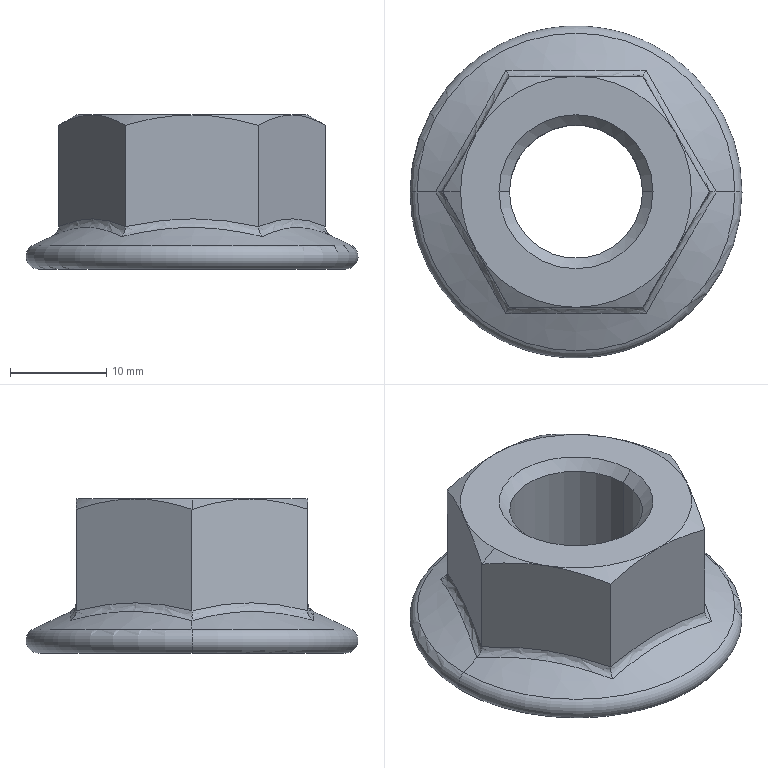Part | STEP file | HEXAGON_NUTS_WITH_FLANGE_GB_GB_ | 1 solid | 31 faces | box 34.5 x 34.5 x 16 mm | volume 6844 mm3 | cone 13 | plane 8 | spline 6 | cylinder 2 | torus 2 | commonest cylinder face diameters 13.835 x2